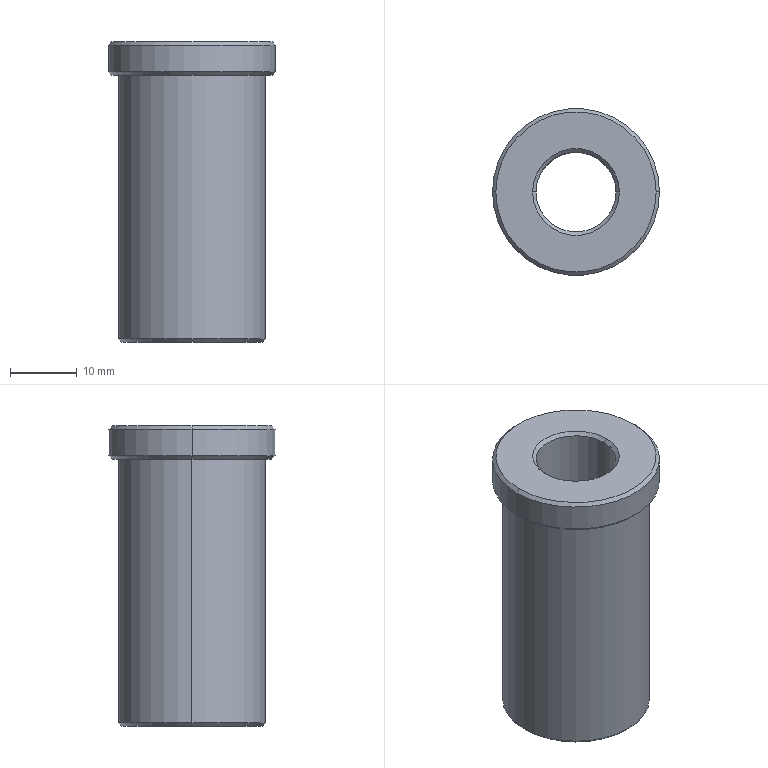Part | STEP file | 1 solid | 19 faces | box 25 x 25 x 45 mm | volume 12533 mm3 | cone 10 | cylinder 6 | plane 3 | commonest cylinder face diameters 12 x2 22 x2 25 x2
STEP:
#1=CARTESIAN_POINT('',(0.,0.,0.));
#2=DIRECTION('',(0.,0.,1.));
#3=DIRECTION('',(1.,0.,0.));
#4=AXIS2_PLACEMENT_3D('',#1,#2,#3);
#5=CARTESIAN_POINT('',(-10.5,0.,-40.));
#6=VERTEX_POINT('',#5);
#7=CARTESIAN_POINT('',(-11.,0.,-39.5));
#8=VERTEX_POINT('',#7);
#9=CARTESIAN_POINT('',(-10.5,0.,-40.));
#10=DIRECTION('',(-0.7071,0.,0.7071));
#11=VECTOR('',#10,1.);
#12=LINE('',#9,#11);
#13=CARTESIAN_POINT('',(0.,0.,-40.));
#14=DIRECTION('',(0.,0.,1.));
#15=DIRECTION('',(1.,0.,0.));
#16=AXIS2_PLACEMENT_3D('',#13,#14,#15);
#17=CONICAL_SURFACE('',#16,10.5,0.7854);
#18=CARTESIAN_POINT('',(3.142,0.));
#19=DIRECTION('',(0.,1.));
#20=VECTOR('',#19,1.);
#21=LINE('',#18,#20);
#22=(GEOMETRIC_REPRESENTATION_CONTEXT(2)PARAMETRIC_REPRESENTATION_CONTEXT()REPRESENTATION_CONTEXT('',''));
#23=DEFINITIONAL_REPRESENTATION('',(#21),#22);
#24=PCURVE('',#17,#23);
#25=CARTESIAN_POINT('',(0.,0.,-40.));
#26=DIRECTION('',(0.,0.,1.));
#27=DIRECTION('',(1.,0.,0.));
#28=AXIS2_PLACEMENT_3D('',#25,#26,#27);
#29=CONICAL_SURFACE('',#28,10.5,0.7854);
#30=CARTESIAN_POINT('',(3.142,0.));
#31=DIRECTION('',(0.,1.));
#32=VECTOR('',#31,1.);
#33=LINE('',#30,#32);
#34=(GEOMETRIC_REPRESENTATION_CONTEXT(2)PARAMETRIC_REPRESENTATION_CONTEXT()REPRESENTATION_CONTEXT('',''));
#35=DEFINITIONAL_REPRESENTATION('',(#33),#34);
#36=PCURVE('',#29,#35);
#37=SURFACE_CURVE('',#12,(#24,#36),.PCURVE_S1.);
#38=EDGE_CURVE('',#6,#8,#37,.T.);
#39=ORIENTED_EDGE('',*,*,#38,.F.);
#40=CARTESIAN_POINT('',(10.5,0.,-40.));
#41=VERTEX_POINT('',#40);
#42=CARTESIAN_POINT('',(0.,0.,-40.));
#43=DIRECTION('',(0.,0.,-1.));
#44=DIRECTION('',(-1.,0.,0.));
#45=AXIS2_PLACEMENT_3D('',#42,#43,#44);
#46=CIRCLE('',#45,10.5);
#47=CARTESIAN_POINT('',(9.425,0.));
#48=DIRECTION('',(-1.,0.));
#49=VECTOR('',#48,1.);
#50=LINE('',#47,#49);
#51=(GEOMETRIC_REPRESENTATION_CONTEXT(2)PARAMETRIC_REPRESENTATION_CONTEXT()REPRESENTATION_CONTEXT('',''));
#52=DEFINITIONAL_REPRESENTATION('',(#50),#51);
#53=PCURVE('',#17,#52);
#54=CARTESIAN_POINT('',(0.,0.,-40.));
#55=DIRECTION('',(0.,0.,-1.));
#56=DIRECTION('',(0.,-1.,0.));
#57=AXIS2_PLACEMENT_3D('',#54,#55,#56);
#58=PLANE('',#57);
#59=CARTESIAN_POINT('',(0.,0.));
#60=DIRECTION('',(0.,1.));
#61=AXIS2_PLACEMENT_2D('',#59,#60);
#62=CIRCLE('',#61,10.5);
#63=(GEOMETRIC_REPRESENTATION_CONTEXT(2)PARAMETRIC_REPRESENTATION_CONTEXT()REPRESENTATION_CONTEXT('',''));
#64=DEFINITIONAL_REPRESENTATION('',(#62),#63);
#65=PCURVE('',#58,#64);
#66=SURFACE_CURVE('',#46,(#53,#65),.PCURVE_S1.);
#67=EDGE_CURVE('',#41,#6,#66,.T.);
#68=ORIENTED_EDGE('',*,*,#67,.F.);
#69=CARTESIAN_POINT('',(11.,0.,-39.5));
#70=VERTEX_POINT('',#69);
#71=CARTESIAN_POINT('',(10.5,0.,-40.));
#72=DIRECTION('',(0.7071,0.,0.7071));
#73=VECTOR('',#72,1.);
#74=LINE('',#71,#73);
#75=CARTESIAN_POINT('',(6.283,0.));
#76=DIRECTION('',(0.,1.));
#77=VECTOR('',#76,1.);
#78=LINE('',#75,#77);
#79=(GEOMETRIC_REPRESENTATION_CONTEXT(2)PARAMETRIC_REPRESENTATION_CONTEXT()REPRESENTATION_CONTEXT('',''));
#80=DEFINITIONAL_REPRESENTATION('',(#78),#79);
#81=PCURVE('',#17,#80);
#82=CARTESIAN_POINT('',(0.,0.));
#83=DIRECTION('',(0.,1.));
#84=VECTOR('',#83,1.);
#85=LINE('',#82,#84);
#86=(GEOMETRIC_REPRESENTATION_CONTEXT(2)PARAMETRIC_REPRESENTATION_CONTEXT()REPRESENTATION_CONTEXT('',''));
#87=DEFINITIONAL_REPRESENTATION('',(#85),#86);
#88=PCURVE('',#29,#87);
#89=SURFACE_CURVE('',#74,(#81,#88),.PCURVE_S1.);
#90=EDGE_CURVE('',#41,#70,#89,.T.);
#91=ORIENTED_EDGE('',*,*,#90,.T.);
#92=CARTESIAN_POINT('',(0.,0.,-39.5));
#93=DIRECTION('',(0.,0.,1.));
#94=DIRECTION('',(-1.,0.,0.));
#95=AXIS2_PLACEMENT_3D('',#92,#93,#94);
#96=CIRCLE('',#95,11.);
#97=CARTESIAN_POINT('',(3.142,0.5));
#98=DIRECTION('',(1.,0.));
#99=VECTOR('',#98,1.);
#100=LINE('',#97,#99);
#101=(GEOMETRIC_REPRESENTATION_CONTEXT(2)PARAMETRIC_REPRESENTATION_CONTEXT()REPRESENTATION_CONTEXT('',''));
#102=DEFINITIONAL_REPRESENTATION('',(#100),#101);
#103=PCURVE('',#17,#102);
#104=CARTESIAN_POINT('',(0.,0.,-40.));
#105=DIRECTION('',(0.,0.,1.));
#106=DIRECTION('',(1.,0.,0.));
#107=AXIS2_PLACEMENT_3D('',#104,#105,#106);
#108=CYLINDRICAL_SURFACE('',#107,11.);
#109=CARTESIAN_POINT('',(3.142,0.5));
#110=DIRECTION('',(1.,0.));
#111=VECTOR('',#110,1.);
#112=LINE('',#109,#111);
#113=(GEOMETRIC_REPRESENTATION_CONTEXT(2)PARAMETRIC_REPRESENTATION_CONTEXT()REPRESENTATION_CONTEXT('',''));
#114=DEFINITIONAL_REPRESENTATION('',(#112),#113);
#115=PCURVE('',#108,#114);
#116=SURFACE_CURVE('',#96,(#103,#115),.PCURVE_S1.);
#117=EDGE_CURVE('',#8,#70,#116,.T.);
#118=ORIENTED_EDGE('',*,*,#117,.F.);
#119=EDGE_LOOP('',(#39,#68,#91,#118));
#120=FACE_BOUND('',#119,.T.);
#121=ADVANCED_FACE('',(#120),#17,.T.);
#122=CARTESIAN_POINT('',(-12.,0.,0.));
#123=VERTEX_POINT('',#122);
#124=CARTESIAN_POINT('',(-12.5,0.,0.5));
#125=VERTEX_POINT('',#124);
#126=CARTESIAN_POINT('',(-12.5,0.,0.5));
#127=DIRECTION('',(-0.7071,0.,0.7071));
#128=VECTOR('',#127,1.);
#129=LINE('',#126,#128);
#130=CARTESIAN_POINT('',(0.,0.,0.5));
#131=DIRECTION('',(0.,0.,1.));
#132=DIRECTION('',(1.,0.,0.));
#133=AXIS2_PLACEMENT_3D('',#130,#131,#132);
#134=CONICAL_SURFACE('',#133,12.5,0.7854);
#135=CARTESIAN_POINT('',(3.142,0.));
#136=DIRECTION('',(0.,1.));
#137=VECTOR('',#136,1.);
#138=LINE('',#135,#137);
#139=(GEOMETRIC_REPRESENTATION_CONTEXT(2)PARAMETRIC_REPRESENTATION_CONTEXT()REPRESENTATION_CONTEXT('',''));
#140=DEFINITIONAL_REPRESENTATION('',(#138),#139);
#141=PCURVE('',#134,#140);
#142=CARTESIAN_POINT('',(0.,0.,0.5));
#143=DIRECTION('',(0.,0.,1.));
#144=DIRECTION('',(1.,0.,0.));
#145=AXIS2_PLACEMENT_3D('',#142,#143,#144);
#146=CONICAL_SURFACE('',#145,12.5,0.7854);
#147=CARTESIAN_POINT('',(3.142,0.));
#148=DIRECTION('',(0.,1.));
#149=VECTOR('',#148,1.);
#150=LINE('',#147,#149);
#151=(GEOMETRIC_REPRESENTATION_CONTEXT(2)PARAMETRIC_REPRESENTATION_CONTEXT()REPRESENTATION_CONTEXT('',''));
#152=DEFINITIONAL_REPRESENTATION('',(#150),#151);
#153=PCURVE('',#146,#152);
#154=SURFACE_CURVE('',#129,(#141,#153),.PCURVE_S1.);
#155=EDGE_CURVE('',#123,#125,#154,.T.);
#156=ORIENTED_EDGE('',*,*,#155,.F.);
#157=CARTESIAN_POINT('',(12.,0.,0.));
#158=VERTEX_POINT('',#157);
#159=CARTESIAN_POINT('',(0.,0.,0.));
#160=DIRECTION('',(0.,0.,-1.));
#161=DIRECTION('',(1.,0.,0.));
#162=AXIS2_PLACEMENT_3D('',#159,#160,#161);
#163=CIRCLE('',#162,12.);
#164=CARTESIAN_POINT('',(6.283,-0.5));
#165=DIRECTION('',(-1.,0.));
#166=VECTOR('',#165,1.);
#167=LINE('',#164,#166);
#168=(GEOMETRIC_REPRESENTATION_CONTEXT(2)PARAMETRIC_REPRESENTATION_CONTEXT()REPRESENTATION_CONTEXT('',''));
#169=DEFINITIONAL_REPRESENTATION('',(#167),#168);
#170=PCURVE('',#134,#169);
#171=CARTESIAN_POINT('',(0.,0.,0.));
#172=DIRECTION('',(0.,0.,1.));
#173=DIRECTION('',(1.,0.,0.));
#174=AXIS2_PLACEMENT_3D('',#171,#172,#173);
#175=PLANE('',#174);
#176=CARTESIAN_POINT('',(12.,0.));
#177=CARTESIAN_POINT('',(12.,-20.785));
#178=CARTESIAN_POINT('',(-6.,-10.392));
#179=CARTESIAN_POINT('',(-24.,0.));
#180=CARTESIAN_POINT('',(-6.,10.392));
#181=CARTESIAN_POINT('',(12.,20.785));
#182=CARTESIAN_POINT('',(12.,0.));
#183=(BOUNDED_CURVE()B_SPLINE_CURVE(2,(#176,#177,#178,#179,#180,#181,#182),.UNSPECIFIED.,.T.,.F.)B_SPLINE_CURVE_WITH_KNOTS((1,2,2,2,2,1),(-2.094,0.,2.094,4.189,6.283,8.378),.UNSPECIFIED.)CURVE()GEOMETRIC_REPRESENTATION_ITEM()RATIONAL_B_SPLINE_CURVE((1.,0.5,1.,0.5,1.,0.5,1.))REPRESENTATION_ITEM(''));
#184=(GEOMETRIC_REPRESENTATION_CONTEXT(2)PARAMETRIC_REPRESENTATION_CONTEXT()REPRESENTATION_CONTEXT('',''));
#185=DEFINITIONAL_REPRESENTATION('',(#183),#184);
#186=PCURVE('',#175,#185);
#187=SURFACE_CURVE('',#163,(#170,#186),.PCURVE_S1.);
#188=EDGE_CURVE('',#158,#123,#187,.T.);
#189=ORIENTED_EDGE('',*,*,#188,.F.);
#190=CARTESIAN_POINT('',(12.5,0.,0.5));
#191=VERTEX_POINT('',#190);
#192=CARTESIAN_POINT('',(12.5,0.,0.5));
#193=DIRECTION('',(0.7071,0.,0.7071));
#194=VECTOR('',#193,1.);
#195=LINE('',#192,#194);
#196=CARTESIAN_POINT('',(6.283,0.));
#197=DIRECTION('',(0.,1.));
#198=VECTOR('',#197,1.);
#199=LINE('',#196,#198);
#200=(GEOMETRIC_REPRESENTATION_CONTEXT(2)PARAMETRIC_REPRESENTATION_CONTEXT()REPRESENTATION_CONTEXT('',''));
#201=DEFINITIONAL_REPRESENTATION('',(#199),#200);
#202=PCURVE('',#134,#201);
#203=CARTESIAN_POINT('',(0.,0.));
#204=DIRECTION('',(0.,1.));
#205=VECTOR('',#204,1.);
#206=LINE('',#203,#205);
#207=(GEOMETRIC_REPRESENTATION_CONTEXT(2)PARAMETRIC_REPRESENTATION_CONTEXT()REPRESENTATION_CONTEXT('',''));
#208=DEFINITIONAL_REPRESENTATION('',(#206),#207);
#209=PCURVE('',#146,#208);
#210=SURFACE_CURVE('',#195,(#202,#209),.PCURVE_S1.);
#211=EDGE_CURVE('',#158,#191,#210,.T.);
#212=ORIENTED_EDGE('',*,*,#211,.T.);
#213=CARTESIAN_POINT('',(0.,0.,0.5));
#214=DIRECTION('',(0.,0.,1.));
#215=DIRECTION('',(1.,0.,0.));
#216=AXIS2_PLACEMENT_3D('',#213,#214,#215);
#217=CIRCLE('',#216,12.5);
#218=CARTESIAN_POINT('',(0.,0.));
#219=DIRECTION('',(1.,0.));
#220=VECTOR('',#219,1.);
#221=LINE('',#218,#220);
#222=(GEOMETRIC_REPRESENTATION_CONTEXT(2)PARAMETRIC_REPRESENTATION_CONTEXT()REPRESENTATION_CONTEXT('',''));
#223=DEFINITIONAL_REPRESENTATION('',(#221),#222);
#224=PCURVE('',#134,#223);
#225=CARTESIAN_POINT('',(0.,0.,5.));
#226=DIRECTION('',(0.,0.,-1.));
#227=DIRECTION('',(-1.,0.,0.));
#228=AXIS2_PLACEMENT_3D('',#225,#226,#227);
#229=CYLINDRICAL_SURFACE('',#228,12.5);
#230=CARTESIAN_POINT('',(9.425,4.5));
#231=DIRECTION('',(-1.,0.));
#232=VECTOR('',#231,1.);
#233=LINE('',#230,#232);
#234=(GEOMETRIC_REPRESENTATION_CONTEXT(2)PARAMETRIC_REPRESENTATION_CONTEXT()REPRESENTATION_CONTEXT('',''));
#235=DEFINITIONAL_REPRESENTATION('',(#233),#234);
#236=PCURVE('',#229,#235);
#237=SURFACE_CURVE('',#217,(#224,#236),.PCURVE_S1.);
#238=EDGE_CURVE('',#125,#191,#237,.T.);
#239=ORIENTED_EDGE('',*,*,#238,.F.);
#240=EDGE_LOOP('',(#156,#189,#212,#239));
#241=FACE_BOUND('',#240,.T.);
#242=ADVANCED_FACE('',(#241),#134,.T.);
#243=CARTESIAN_POINT('',(-6.5,0.,5.));
#244=VERTEX_POINT('',#243);
#245=CARTESIAN_POINT('',(6.5,0.,5.));
#246=VERTEX_POINT('',#245);
#247=CARTESIAN_POINT('',(0.,0.,5.));
#248=DIRECTION('',(0.,0.,-1.));
#249=DIRECTION('',(1.,0.,0.));
#250=AXIS2_PLACEMENT_3D('',#247,#248,#249);
#251=CIRCLE('',#250,6.5);
#252=CARTESIAN_POINT('',(0.,0.,4.5));
#253=DIRECTION('',(0.,0.,1.));
#254=DIRECTION('',(1.,0.,0.));
#255=AXIS2_PLACEMENT_3D('',#252,#253,#254);
#256=CONICAL_SURFACE('',#255,6.,0.7854);
#257=CARTESIAN_POINT('',(6.283,0.5));
#258=DIRECTION('',(-1.,0.));
#259=VECTOR('',#258,1.);
#260=LINE('',#257,#259);
#261=(GEOMETRIC_REPRESENTATION_CONTEXT(2)PARAMETRIC_REPRESENTATION_CONTEXT()REPRESENTATION_CONTEXT('',''));
#262=DEFINITIONAL_REPRESENTATION('',(#260),#261);
#263=PCURVE('',#256,#262);
#264=CARTESIAN_POINT('',(0.,0.,5.));
#265=DIRECTION('',(0.,0.,1.));
#266=DIRECTION('',(1.,0.,0.));
#267=AXIS2_PLACEMENT_3D('',#264,#265,#266);
#268=PLANE('',#267);
#269=CARTESIAN_POINT('',(6.5,0.));
#270=CARTESIAN_POINT('',(6.5,-11.258));
#271=CARTESIAN_POINT('',(-3.25,-5.629));
#272=CARTESIAN_POINT('',(-13.,0.));
#273=CARTESIAN_POINT('',(-3.25,5.629));
#274=CARTESIAN_POINT('',(6.5,11.258));
#275=CARTESIAN_POINT('',(6.5,0.));
#276=(BOUNDED_CURVE()B_SPLINE_CURVE(2,(#269,#270,#271,#272,#273,#274,#275),.UNSPECIFIED.,.T.,.F.)B_SPLINE_CURVE_WITH_KNOTS((1,2,2,2,2,1),(-2.094,0.,2.094,4.189,6.283,8.378),.UNSPECIFIED.)CURVE()GEOMETRIC_REPRESENTATION_ITEM()RATIONAL_B_SPLINE_CURVE((1.,0.5,1.,0.5,1.,0.5,1.))REPRESENTATION_ITEM(''));
#277=(GEOMETRIC_REPRESENTATION_CONTEXT(2)PARAMETRIC_REPRESENTATION_CONTEXT()REPRESENTATION_CONTEXT('',''));
#278=DEFINITIONAL_REPRESENTATION('',(#276),#277);
#279=PCURVE('',#268,#278);
#280=SURFACE_CURVE('',#251,(#263,#279),.PCURVE_S1.);
#281=EDGE_CURVE('',#244,#246,#280,.T.);
#282=ORIENTED_EDGE('',*,*,#281,.T.);
#283=CARTESIAN_POINT('',(6.,0.,4.5));
#284=VERTEX_POINT('',#283);
#285=CARTESIAN_POINT('',(6.,0.,4.5));
#286=DIRECTION('',(0.7071,0.,0.7071));
#287=VECTOR('',#286,1.);
#288=LINE('',#285,#287);
#289=CARTESIAN_POINT('',(0.,0.));
#290=DIRECTION('',(0.,1.));
#291=VECTOR('',#290,1.);
#292=LINE('',#289,#291);
#293=(GEOMETRIC_REPRESENTATION_CONTEXT(2)PARAMETRIC_REPRESENTATION_CONTEXT()REPRESENTATION_CONTEXT('',''));
#294=DEFINITIONAL_REPRESENTATION('',(#292),#293);
#295=PCURVE('',#256,#294);
#296=CARTESIAN_POINT('',(0.,0.,4.5));
#297=DIRECTION('',(0.,0.,1.));
#298=DIRECTION('',(1.,0.,0.));
#299=AXIS2_PLACEMENT_3D('',#296,#297,#298);
#300=CONICAL_SURFACE('',#299,6.,0.7854);
#301=CARTESIAN_POINT('',(6.283,0.));
#302=DIRECTION('',(0.,1.));
#303=VECTOR('',#302,1.);
#304=LINE('',#301,#303);
#305=(GEOMETRIC_REPRESENTATION_CONTEXT(2)PARAMETRIC_REPRESENTATION_CONTEXT()REPRESENTATION_CONTEXT('',''));
#306=DEFINITIONAL_REPRESENTATION('',(#304),#305);
#307=PCURVE('',#300,#306);
#308=SURFACE_CURVE('',#288,(#295,#307),.PCURVE_S1.);
#309=EDGE_CURVE('',#284,#246,#308,.T.);
#310=ORIENTED_EDGE('',*,*,#309,.F.);
#311=CARTESIAN_POINT('',(-6.,0.,4.5));
#312=VERTEX_POINT('',#311);
#313=CARTESIAN_POINT('',(0.,0.,4.5));
#314=DIRECTION('',(0.,0.,1.));
#315=DIRECTION('',(1.,0.,0.));
#316=AXIS2_PLACEMENT_3D('',#313,#314,#315);
#317=CIRCLE('',#316,6.);
#318=CARTESIAN_POINT('',(0.,0.));
#319=DIRECTION('',(1.,0.));
#320=VECTOR('',#319,1.);
#321=LINE('',#318,#320);
#322=(GEOMETRIC_REPRESENTATION_CONTEXT(2)PARAMETRIC_REPRESENTATION_CONTEXT()REPRESENTATION_CONTEXT('',''));
#323=DEFINITIONAL_REPRESENTATION('',(#321),#322);
#324=PCURVE('',#256,#323);
#325=CARTESIAN_POINT('',(0.,0.,5.));
#326=DIRECTION('',(0.,0.,-1.));
#327=DIRECTION('',(-1.,0.,0.));
#328=AXIS2_PLACEMENT_3D('',#325,#326,#327);
#329=CYLINDRICAL_SURFACE('',#328,6.);
#330=CARTESIAN_POINT('',(3.142,0.5));
#331=DIRECTION('',(-1.,0.));
#332=VECTOR('',#331,1.);
#333=LINE('',#330,#332);
#334=(GEOMETRIC_REPRESENTATION_CONTEXT(2)PARAMETRIC_REPRESENTATION_CONTEXT()REPRESENTATION_CONTEXT('',''));
#335=DEFINITIONAL_REPRESENTATION('',(#333),#334);
#336=PCURVE('',#329,#335);
#337=SURFACE_CURVE('',#317,(#324,#336),.PCURVE_S1.);
#338=EDGE_CURVE('',#284,#312,#337,.T.);
#339=ORIENTED_EDGE('',*,*,#338,.T.);
#340=CARTESIAN_POINT('',(-6.,0.,4.5));
#341=DIRECTION('',(-0.7071,0.,0.7071));
#342=VECTOR('',#341,1.);
#343=LINE('',#340,#342);
#344=CARTESIAN_POINT('',(3.142,0.));
#345=DIRECTION('',(0.,1.));
#346=VECTOR('',#345,1.);
#347=LINE('',#344,#346);
#348=(GEOMETRIC_REPRESENTATION_CONTEXT(2)PARAMETRIC_REPRESENTATION_CONTEXT()REPRESENTATION_CONTEXT('',''));
#349=DEFINITIONAL_REPRESENTATION('',(#347),#348);
#350=PCURVE('',#256,#349);
#351=CARTESIAN_POINT('',(3.142,0.));
#352=DIRECTION('',(0.,1.));
#353=VECTOR('',#352,1.);
#354=LINE('',#351,#353);
#355=(GEOMETRIC_REPRESENTATION_CONTEXT(2)PARAMETRIC_REPRESENTATION_CONTEXT()REPRESENTATION_CONTEXT('',''));
#356=DEFINITIONAL_REPRESENTATION('',(#354),#355);
#357=PCURVE('',#300,#356);
#358=SURFACE_CURVE('',#343,(#350,#357),.PCURVE_S1.);
#359=EDGE_CURVE('',#312,#244,#358,.T.);
#360=ORIENTED_EDGE('',*,*,#359,.T.);
#361=EDGE_LOOP('',(#282,#310,#339,#360));
#362=FACE_BOUND('',#361,.F.);
#363=ADVANCED_FACE('',(#362),#256,.F.);
#364=CARTESIAN_POINT('',(6.5,0.,-40.));
#365=VERTEX_POINT('',#364);
#366=CARTESIAN_POINT('',(-6.5,0.,-40.));
#367=VERTEX_POINT('',#366);
#368=CARTESIAN_POINT('',(0.,0.,-40.));
#369=DIRECTION('',(0.,0.,1.));
#370=DIRECTION('',(-1.,0.,0.));
#371=AXIS2_PLACEMENT_3D('',#368,#369,#370);
#372=CIRCLE('',#371,6.5);
#373=CARTESIAN_POINT('',(0.,0.,-39.5));
#374=DIRECTION('',(0.,0.,-1.));
#375=DIRECTION('',(-1.,0.,0.));
#376=AXIS2_PLACEMENT_3D('',#373,#374,#375);
#377=CONICAL_SURFACE('',#376,6.,0.7854);
#378=CARTESIAN_POINT('',(6.283,0.5));
#379=DIRECTION('',(-1.,0.));
#380=VECTOR('',#379,1.);
#381=LINE('',#378,#380);
#382=(GEOMETRIC_REPRESENTATION_CONTEXT(2)PARAMETRIC_REPRESENTATION_CONTEXT()REPRESENTATION_CONTEXT('',''));
#383=DEFINITIONAL_REPRESENTATION('',(#381),#382);
#384=PCURVE('',#377,#383);
#385=CARTESIAN_POINT('',(0.,6.5));
#386=CARTESIAN_POINT('',(11.258,6.5));
#387=CARTESIAN_POINT('',(5.629,-3.25));
#388=CARTESIAN_POINT('',(0.,-13.));
#389=CARTESIAN_POINT('',(-5.629,-3.25));
#390=CARTESIAN_POINT('',(-11.258,6.5));
#391=CARTESIAN_POINT('',(0.,6.5));
#392=(BOUNDED_CURVE()B_SPLINE_CURVE(2,(#385,#386,#387,#388,#389,#390,#391),.UNSPECIFIED.,.T.,.F.)B_SPLINE_CURVE_WITH_KNOTS((1,2,2,2,2,1),(-2.094,0.,2.094,4.189,6.283,8.378),.UNSPECIFIED.)CURVE()GEOMETRIC_REPRESENTATION_ITEM()RATIONAL_B_SPLINE_CURVE((1.,0.5,1.,0.5,1.,0.5,1.))REPRESENTATION_ITEM(''));
#393=(GEOMETRIC_REPRESENTATION_CONTEXT(2)PARAMETRIC_REPRESENTATION_CONTEXT()REPRESENTATION_CONTEXT('',''));
#394=DEFINITIONAL_REPRESENTATION('',(#392),#393);
#395=PCURVE('',#58,#394);
#396=SURFACE_CURVE('',#372,(#384,#395),.PCURVE_S1.);
#397=EDGE_CURVE('',#365,#367,#396,.T.);
#398=ORIENTED_EDGE('',*,*,#397,.T.);
#399=CARTESIAN_POINT('',(-6.,0.,-39.5));
#400=VERTEX_POINT('',#399);
#401=CARTESIAN_POINT('',(-6.,0.,-39.5));
#402=DIRECTION('',(-0.7071,0.,-0.7071));
#403=VECTOR('',#402,1.);
#404=LINE('',#401,#403);
#405=CARTESIAN_POINT('',(0.,0.));
#406=DIRECTION('',(0.,1.));
#407=VECTOR('',#406,1.);
#408=LINE('',#405,#407);
#409=(GEOMETRIC_REPRESENTATION_CONTEXT(2)PARAMETRIC_REPRESENTATION_CONTEXT()REPRESENTATION_CONTEXT('',''));
#410=DEFINITIONAL_REPRESENTATION('',(#408),#409);
#411=PCURVE('',#377,#410);
#412=CARTESIAN_POINT('',(0.,0.,-39.5));
#413=DIRECTION('',(0.,0.,-1.));
#414=DIRECTION('',(-1.,0.,0.));
#415=AXIS2_PLACEMENT_3D('',#412,#413,#414);
#416=CONICAL_SURFACE('',#415,6.,0.7854);
#417=CARTESIAN_POINT('',(6.283,0.));
#418=DIRECTION('',(0.,1.));
#419=VECTOR('',#418,1.);
#420=LINE('',#417,#419);
#421=(GEOMETRIC_REPRESENTATION_CONTEXT(2)PARAMETRIC_REPRESENTATION_CONTEXT()REPRESENTATION_CONTEXT('',''));
#422=DEFINITIONAL_REPRESENTATION('',(#420),#421);
#423=PCURVE('',#416,#422);
#424=SURFACE_CURVE('',#404,(#411,#423),.PCURVE_S1.);
#425=EDGE_CURVE('',#400,#367,#424,.T.);
#426=ORIENTED_EDGE('',*,*,#425,.F.);
#427=CARTESIAN_POINT('',(6.,0.,-39.5));
#428=VERTEX_POINT('',#427);
#429=CARTESIAN_POINT('',(0.,0.,-39.5));
#430=DIRECTION('',(0.,0.,-1.));
#431=DIRECTION('',(-1.,0.,0.));
#432=AXIS2_PLACEMENT_3D('',#429,#430,#431);
#433=CIRCLE('',#432,6.);
#434=CARTESIAN_POINT('',(0.,0.));
#435=DIRECTION('',(1.,0.));
#436=VECTOR('',#435,1.);
#437=LINE('',#434,#436);
#438=(GEOMETRIC_REPRESENTATION_CONTEXT(2)PARAMETRIC_REPRESENTATION_CONTEXT()REPRESENTATION_CONTEXT('',''));
#439=DEFINITIONAL_REPRESENTATION('',(#437),#438);
#440=PCURVE('',#377,#439);
#441=CARTESIAN_POINT('',(0.,44.5));
#442=DIRECTION('',(1.,0.));
#443=VECTOR('',#442,1.);
#444=LINE('',#441,#443);
#445=(GEOMETRIC_REPRESENTATION_CONTEXT(2)PARAMETRIC_REPRESENTATION_CONTEXT()REPRESENTATION_CONTEXT('',''));
#446=DEFINITIONAL_REPRESENTATION('',(#444),#445);
#447=PCURVE('',#329,#446);
#448=SURFACE_CURVE('',#433,(#440,#447),.PCURVE_S1.);
#449=EDGE_CURVE('',#400,#428,#448,.T.);
#450=ORIENTED_EDGE('',*,*,#449,.T.);
#451=CARTESIAN_POINT('',(6.,0.,-39.5));
#452=DIRECTION('',(0.7071,0.,-0.7071));
#453=VECTOR('',#452,1.);
#454=LINE('',#451,#453);
#455=CARTESIAN_POINT('',(3.142,0.));
#456=DIRECTION('',(0.,1.));
#457=VECTOR('',#456,1.);
#458=LINE('',#455,#457);
#459=(GEOMETRIC_REPRESENTATION_CONTEXT(2)PARAMETRIC_REPRESENTATION_CONTEXT()REPRESENTATION_CONTEXT('',''));
#460=DEFINITIONAL_REPRESENTATION('',(#458),#459);
#461=PCURVE('',#377,#460);
#462=CARTESIAN_POINT('',(3.142,0.));
#463=DIRECTION('',(0.,1.));
#464=VECTOR('',#463,1.);
#465=LINE('',#462,#464);
#466=(GEOMETRIC_REPRESENTATION_CONTEXT(2)PARAMETRIC_REPRESENTATION_CONTEXT()REPRESENTATION_CONTEXT('',''));
#467=DEFINITIONAL_REPRESENTATION('',(#465),#466);
#468=PCURVE('',#416,#467);
#469=SURFACE_CURVE('',#454,(#461,#468),.PCURVE_S1.);
#470=EDGE_CURVE('',#428,#365,#469,.T.);
#471=ORIENTED_EDGE('',*,*,#470,.T.);
#472=EDGE_LOOP('',(#398,#426,#450,#471));
#473=FACE_BOUND('',#472,.F.);
#474=ADVANCED_FACE('',(#473),#377,.F.);
#475=CARTESIAN_POINT('',(12.,0.,5.));
#476=VERTEX_POINT('',#475);
#477=CARTESIAN_POINT('',(12.5,0.,4.5));
#478=VERTEX_POINT('',#477);
#479=CARTESIAN_POINT('',(12.,0.,5.));
#480=DIRECTION('',(0.7071,0.,-0.7071));
#481=VECTOR('',#480,1.);
#482=LINE('',#479,#481);
#483=CARTESIAN_POINT('',(0.,0.,5.));
#484=DIRECTION('',(0.,0.,-1.));
#485=DIRECTION('',(-1.,0.,0.));
#486=AXIS2_PLACEMENT_3D('',#483,#484,#485);
#487=CONICAL_SURFACE('',#486,12.,0.7854);
#488=CARTESIAN_POINT('',(3.142,0.));
#489=DIRECTION('',(0.,1.));
#490=VECTOR('',#489,1.);
#491=LINE('',#488,#490);
#492=(GEOMETRIC_REPRESENTATION_CONTEXT(2)PARAMETRIC_REPRESENTATION_CONTEXT()REPRESENTATION_CONTEXT('',''));
#493=DEFINITIONAL_REPRESENTATION('',(#491),#492);
#494=PCURVE('',#487,#493);
#495=CARTESIAN_POINT('',(0.,0.,5.));
#496=DIRECTION('',(0.,0.,-1.));
#497=DIRECTION('',(-1.,0.,0.));
#498=AXIS2_PLACEMENT_3D('',#495,#496,#497);
#499=CONICAL_SURFACE('',#498,12.,0.7854);
#500=CARTESIAN_POINT('',(3.142,0.));
#501=DIRECTION('',(0.,1.));
#502=VECTOR('',#501,1.);
#503=LINE('',#500,#502);
#504=(GEOMETRIC_REPRESENTATION_CONTEXT(2)PARAMETRIC_REPRESENTATION_CONTEXT()REPRESENTATION_CONTEXT('',''));
#505=DEFINITIONAL_REPRESENTATION('',(#503),#504);
#506=PCURVE('',#499,#505);
#507=SURFACE_CURVE('',#482,(#494,#506),.PCURVE_S1.);
#508=EDGE_CURVE('',#476,#478,#507,.T.);
#509=ORIENTED_EDGE('',*,*,#508,.F.);
#510=CARTESIAN_POINT('',(-12.,0.,5.));
#511=VERTEX_POINT('',#510);
#512=CARTESIAN_POINT('',(0.,0.,5.));
#513=DIRECTION('',(0.,0.,1.));
#514=DIRECTION('',(1.,0.,0.));
#515=AXIS2_PLACEMENT_3D('',#512,#513,#514);
#516=CIRCLE('',#515,12.);
#517=CARTESIAN_POINT('',(9.425,0.));
#518=DIRECTION('',(-1.,0.));
#519=VECTOR('',#518,1.);
#520=LINE('',#517,#519);
#521=(GEOMETRIC_REPRESENTATION_CONTEXT(2)PARAMETRIC_REPRESENTATION_CONTEXT()REPRESENTATION_CONTEXT('',''));
#522=DEFINITIONAL_REPRESENTATION('',(#520),#521);
#523=PCURVE('',#487,#522);
#524=CARTESIAN_POINT('',(0.,0.));
#525=DIRECTION('',(1.,0.));
#526=AXIS2_PLACEMENT_2D('',#524,#525);
#527=CIRCLE('',#526,12.);
#528=(GEOMETRIC_REPRESENTATION_CONTEXT(2)PARAMETRIC_REPRESENTATION_CONTEXT()REPRESENTATION_CONTEXT('',''));
#529=DEFINITIONAL_REPRESENTATION('',(#527),#528);
#530=PCURVE('',#268,#529);
#531=SURFACE_CURVE('',#516,(#523,#530),.PCURVE_S1.);
#532=EDGE_CURVE('',#511,#476,#531,.T.);
#533=ORIENTED_EDGE('',*,*,#532,.F.);
#534=CARTESIAN_POINT('',(-12.5,0.,4.5));
#535=VERTEX_POINT('',#534);
#536=CARTESIAN_POINT('',(-12.,0.,5.));
#537=DIRECTION('',(-0.7071,0.,-0.7071));
#538=VECTOR('',#537,1.);
#539=LINE('',#536,#538);
#540=CARTESIAN_POINT('',(6.283,0.));
#541=DIRECTION('',(0.,1.));
#542=VECTOR('',#541,1.);
#543=LINE('',#540,#542);
#544=(GEOMETRIC_REPRESENTATION_CONTEXT(2)PARAMETRIC_REPRESENTATION_CONTEXT()REPRESENTATION_CONTEXT('',''));
#545=DEFINITIONAL_REPRESENTATION('',(#543),#544);
#546=PCURVE('',#487,#545);
#547=CARTESIAN_POINT('',(0.,0.));
#548=DIRECTION('',(0.,1.));
#549=VECTOR('',#548,1.);
#550=LINE('',#547,#549);
#551=(GEOMETRIC_REPRESENTATION_CONTEXT(2)PARAMETRIC_REPRESENTATION_CONTEXT()REPRESENTATION_CONTEXT('',''));
#552=DEFINITIONAL_REPRESENTATION('',(#550),#551);
#553=PCURVE('',#499,#552);
#554=SURFACE_CURVE('',#539,(#546,#553),.PCURVE_S1.);
#555=EDGE_CURVE('',#511,#535,#554,.T.);
#556=ORIENTED_EDGE('',*,*,#555,.T.);
#557=CARTESIAN_POINT('',(0.,0.,4.5));
#558=DIRECTION('',(0.,0.,-1.));
#559=DIRECTION('',(1.,0.,0.));
#560=AXIS2_PLACEMENT_3D('',#557,#558,#559);
#561=CIRCLE('',#560,12.5);
#562=CARTESIAN_POINT('',(3.142,0.5));
#563=DIRECTION('',(1.,0.));
#564=VECTOR('',#563,1.);
#565=LINE('',#562,#564);
#566=(GEOMETRIC_REPRESENTATION_CONTEXT(2)PARAMETRIC_REPRESENTATION_CONTEXT()REPRESENTATION_CONTEXT('',''));
#567=DEFINITIONAL_REPRESENTATION('',(#565),#566);
#568=PCURVE('',#487,#567);
#569=CARTESIAN_POINT('',(3.142,0.5));
#570=DIRECTION('',(1.,0.));
#571=VECTOR('',#570,1.);
#572=LINE('',#569,#571);
#573=(GEOMETRIC_REPRESENTATION_CONTEXT(2)PARAMETRIC_REPRESENTATION_CONTEXT()REPRESENTATION_CONTEXT('',''));
#574=DEFINITIONAL_REPRESENTATION('',(#572),#573);
#575=PCURVE('',#229,#574);
#576=SURFACE_CURVE('',#561,(#568,#575),.PCURVE_S1.);
#577=EDGE_CURVE('',#478,#535,#576,.T.);
#578=ORIENTED_EDGE('',*,*,#577,.F.);
#579=EDGE_LOOP('',(#509,#533,#556,#578));
#580=FACE_BOUND('',#579,.T.);
#581=ADVANCED_FACE('',(#580),#487,.T.);
#582=CARTESIAN_POINT('',(-11.,0.,0.));
#583=VERTEX_POINT('',#582);
#584=CARTESIAN_POINT('',(-11.,0.,-40.));
#585=DIRECTION('',(0.,0.,1.));
#586=VECTOR('',#585,1.);
#587=LINE('',#584,#586);
#588=CARTESIAN_POINT('',(3.142,0.));
#589=DIRECTION('',(0.,1.));
#590=VECTOR('',#589,1.);
#591=LINE('',#588,#590);
#592=(GEOMETRIC_REPRESENTATION_CONTEXT(2)PARAMETRIC_REPRESENTATION_CONTEXT()REPRESENTATION_CONTEXT('',''));
#593=DEFINITIONAL_REPRESENTATION('',(#591),#592);
#594=PCURVE('',#108,#593);
#595=CARTESIAN_POINT('',(0.,0.,-40.));
#596=DIRECTION('',(0.,0.,1.));
#597=DIRECTION('',(1.,0.,0.));
#598=AXIS2_PLACEMENT_3D('',#595,#596,#597);
#599=CYLINDRICAL_SURFACE('',#598,11.);
#600=CARTESIAN_POINT('',(3.142,0.));
#601=DIRECTION('',(0.,1.));
#602=VECTOR('',#601,1.);
#603=LINE('',#600,#602);
#604=(GEOMETRIC_REPRESENTATION_CONTEXT(2)PARAMETRIC_REPRESENTATION_CONTEXT()REPRESENTATION_CONTEXT('',''));
#605=DEFINITIONAL_REPRESENTATION('',(#603),#604);
#606=PCURVE('',#599,#605);
#607=SURFACE_CURVE('',#587,(#594,#606),.PCURVE_S1.);
#608=EDGE_CURVE('',#8,#583,#607,.T.);
#609=ORIENTED_EDGE('',*,*,#608,.F.);
#610=ORIENTED_EDGE('',*,*,#117,.T.);
#611=CARTESIAN_POINT('',(11.,0.,0.));
#612=VERTEX_POINT('',#611);
#613=CARTESIAN_POINT('',(11.,0.,-40.));
#614=DIRECTION('',(0.,0.,1.));
#615=VECTOR('',#614,1.);
#616=LINE('',#613,#615);
#617=CARTESIAN_POINT('',(6.283,0.));
#618=DIRECTION('',(0.,1.));
#619=VECTOR('',#618,1.);
#620=LINE('',#617,#619);
#621=(GEOMETRIC_REPRESENTATION_CONTEXT(2)PARAMETRIC_REPRESENTATION_CONTEXT()REPRESENTATION_CONTEXT('',''));
#622=DEFINITIONAL_REPRESENTATION('',(#620),#621);
#623=PCURVE('',#108,#622);
#624=CARTESIAN_POINT('',(0.,0.));
#625=DIRECTION('',(0.,1.));
#626=VECTOR('',#625,1.);
#627=LINE('',#624,#626);
#628=(GEOMETRIC_REPRESENTATION_CONTEXT(2)PARAMETRIC_REPRESENTATION_CONTEXT()REPRESENTATION_CONTEXT('',''));
#629=DEFINITIONAL_REPRESENTATION('',(#627),#628);
#630=PCURVE('',#599,#629);
#631=SURFACE_CURVE('',#616,(#623,#630),.PCURVE_S1.);
#632=EDGE_CURVE('',#70,#612,#631,.T.);
#633=ORIENTED_EDGE('',*,*,#632,.T.);
#634=CARTESIAN_POINT('',(0.,0.,0.));
#635=DIRECTION('',(0.,0.,-1.));
#636=DIRECTION('',(-1.,0.,0.));
#637=AXIS2_PLACEMENT_3D('',#634,#635,#636);
#638=CIRCLE('',#637,11.);
#639=CARTESIAN_POINT('',(9.425,40.));
#640=DIRECTION('',(-1.,0.));
#641=VECTOR('',#640,1.);
#642=LINE('',#639,#641);
#643=(GEOMETRIC_REPRESENTATION_CONTEXT(2)PARAMETRIC_REPRESENTATION_CONTEXT()REPRESENTATION_CONTEXT('',''));
#644=DEFINITIONAL_REPRESENTATION('',(#642),#643);
#645=PCURVE('',#108,#644);
#646=CARTESIAN_POINT('',(-11.,0.));
#647=CARTESIAN_POINT('',(-11.,19.053));
#648=CARTESIAN_POINT('',(5.5,9.526));
#649=CARTESIAN_POINT('',(22.,0.));
#650=CARTESIAN_POINT('',(5.5,-9.526));
#651=CARTESIAN_POINT('',(-11.,-19.053));
#652=CARTESIAN_POINT('',(-11.,0.));
#653=(BOUNDED_CURVE()B_SPLINE_CURVE(2,(#646,#647,#648,#649,#650,#651,#652),.UNSPECIFIED.,.T.,.F.)B_SPLINE_CURVE_WITH_KNOTS((1,2,2,2,2,1),(-2.094,0.,2.094,4.189,6.283,8.378),.UNSPECIFIED.)CURVE()GEOMETRIC_REPRESENTATION_ITEM()RATIONAL_B_SPLINE_CURVE((1.,0.5,1.,0.5,1.,0.5,1.))REPRESENTATION_ITEM(''));
#654=(GEOMETRIC_REPRESENTATION_CONTEXT(2)PARAMETRIC_REPRESENTATION_CONTEXT()REPRESENTATION_CONTEXT('',''));
#655=DEFINITIONAL_REPRESENTATION('',(#653),#654);
#656=PCURVE('',#175,#655);
#657=SURFACE_CURVE('',#638,(#645,#656),.PCURVE_S1.);
#658=EDGE_CURVE('',#612,#583,#657,.T.);
#659=ORIENTED_EDGE('',*,*,#658,.T.);
#660=EDGE_LOOP('',(#609,#610,#633,#659));
#661=FACE_BOUND('',#660,.T.);
#662=ADVANCED_FACE('',(#661),#108,.T.);
#663=CARTESIAN_POINT('',(0.,0.,-40.));
#664=DIRECTION('',(0.,0.,1.));
#665=DIRECTION('',(-1.,0.,0.));
#666=AXIS2_PLACEMENT_3D('',#663,#664,#665);
#667=CIRCLE('',#666,6.5);
#668=CARTESIAN_POINT('',(0.,6.5));
#669=CARTESIAN_POINT('',(11.258,6.5));
#670=CARTESIAN_POINT('',(5.629,-3.25));
#671=CARTESIAN_POINT('',(0.,-13.));
#672=CARTESIAN_POINT('',(-5.629,-3.25));
#673=CARTESIAN_POINT('',(-11.258,6.5));
#674=CARTESIAN_POINT('',(0.,6.5));
#675=(BOUNDED_CURVE()B_SPLINE_CURVE(2,(#668,#669,#670,#671,#672,#673,#674),.UNSPECIFIED.,.T.,.F.)B_SPLINE_CURVE_WITH_KNOTS((1,2,2,2,2,1),(-2.094,0.,2.094,4.189,6.283,8.378),.UNSPECIFIED.)CURVE()GEOMETRIC_REPRESENTATION_ITEM()RATIONAL_B_SPLINE_CURVE((1.,0.5,1.,0.5,1.,0.5,1.))REPRESENTATION_ITEM(''));
#676=(GEOMETRIC_REPRESENTATION_CONTEXT(2)PARAMETRIC_REPRESENTATION_CONTEXT()REPRESENTATION_CONTEXT('',''));
#677=DEFINITIONAL_REPRESENTATION('',(#675),#676);
#678=PCURVE('',#58,#677);
#679=CARTESIAN_POINT('',(6.283,0.5));
#680=DIRECTION('',(-1.,0.));
#681=VECTOR('',#680,1.);
#682=LINE('',#679,#681);
#683=(GEOMETRIC_REPRESENTATION_CONTEXT(2)PARAMETRIC_REPRESENTATION_CONTEXT()REPRESENTATION_CONTEXT('',''));
#684=DEFINITIONAL_REPRESENTATION('',(#682),#683);
#685=PCURVE('',#416,#684);
#686=SURFACE_CURVE('',#667,(#678,#685),.PCURVE_S1.);
#687=EDGE_CURVE('',#367,#365,#686,.T.);
#688=ORIENTED_EDGE('',*,*,#687,.T.);
#689=ORIENTED_EDGE('',*,*,#397,.T.);
#690=EDGE_LOOP('',(#688,#689));
#691=FACE_BOUND('',#690,.T.);
#692=ORIENTED_EDGE('',*,*,#67,.T.);
#693=CARTESIAN_POINT('',(0.,0.,-40.));
#694=DIRECTION('',(0.,0.,-1.));
#695=DIRECTION('',(-1.,0.,0.));
#696=AXIS2_PLACEMENT_3D('',#693,#694,#695);
#697=CIRCLE('',#696,10.5);
#698=CARTESIAN_POINT('',(0.,0.));
#699=DIRECTION('',(0.,1.));
#700=AXIS2_PLACEMENT_2D('',#698,#699);
#701=CIRCLE('',#700,10.5);
#702=(GEOMETRIC_REPRESENTATION_CONTEXT(2)PARAMETRIC_REPRESENTATION_CONTEXT()REPRESENTATION_CONTEXT('',''));
#703=DEFINITIONAL_REPRESENTATION('',(#701),#702);
#704=PCURVE('',#58,#703);
#705=CARTESIAN_POINT('',(3.142,0.));
#706=DIRECTION('',(-1.,0.));
#707=VECTOR('',#706,1.);
#708=LINE('',#705,#707);
#709=(GEOMETRIC_REPRESENTATION_CONTEXT(2)PARAMETRIC_REPRESENTATION_CONTEXT()REPRESENTATION_CONTEXT('',''));
#710=DEFINITIONAL_REPRESENTATION('',(#708),#709);
#711=PCURVE('',#29,#710);
#712=SURFACE_CURVE('',#697,(#704,#711),.PCURVE_S1.);
#713=EDGE_CURVE('',#6,#41,#712,.T.);
#714=ORIENTED_EDGE('',*,*,#713,.T.);
#715=EDGE_LOOP('',(#692,#714));
#716=FACE_BOUND('',#715,.T.);
#717=ADVANCED_FACE('',(#691,#716),#58,.T.);
#718=ORIENTED_EDGE('',*,*,#449,.F.);
#719=CARTESIAN_POINT('',(-6.,0.,5.));
#720=DIRECTION('',(0.,0.,-1.));
#721=VECTOR('',#720,1.);
#722=LINE('',#719,#721);
#723=CARTESIAN_POINT('',(0.,0.));
#724=DIRECTION('',(0.,1.));
#725=VECTOR('',#724,1.);
#726=LINE('',#723,#725);
#727=(GEOMETRIC_REPRESENTATION_CONTEXT(2)PARAMETRIC_REPRESENTATION_CONTEXT()REPRESENTATION_CONTEXT('',''));
#728=DEFINITIONAL_REPRESENTATION('',(#726),#727);
#729=PCURVE('',#329,#728);
#730=CARTESIAN_POINT('',(0.,0.,5.));
#731=DIRECTION('',(0.,0.,-1.));
#732=DIRECTION('',(-1.,0.,0.));
#733=AXIS2_PLACEMENT_3D('',#730,#731,#732);
#734=CYLINDRICAL_SURFACE('',#733,6.);
#735=CARTESIAN_POINT('',(6.283,0.));
#736=DIRECTION('',(0.,1.));
#737=VECTOR('',#736,1.);
#738=LINE('',#735,#737);
#739=(GEOMETRIC_REPRESENTATION_CONTEXT(2)PARAMETRIC_REPRESENTATION_CONTEXT()REPRESENTATION_CONTEXT('',''));
#740=DEFINITIONAL_REPRESENTATION('',(#738),#739);
#741=PCURVE('',#734,#740);
#742=SURFACE_CURVE('',#722,(#729,#741),.PCURVE_S1.);
#743=EDGE_CURVE('',#312,#400,#742,.T.);
#744=ORIENTED_EDGE('',*,*,#743,.F.);
#745=ORIENTED_EDGE('',*,*,#338,.F.);
#746=CARTESIAN_POINT('',(6.,0.,5.));
#747=DIRECTION('',(0.,0.,-1.));
#748=VECTOR('',#747,1.);
#749=LINE('',#746,#748);
#750=CARTESIAN_POINT('',(3.142,0.));
#751=DIRECTION('',(0.,1.));
#752=VECTOR('',#751,1.);
#753=LINE('',#750,#752);
#754=(GEOMETRIC_REPRESENTATION_CONTEXT(2)PARAMETRIC_REPRESENTATION_CONTEXT()REPRESENTATION_CONTEXT('',''));
#755=DEFINITIONAL_REPRESENTATION('',(#753),#754);
#756=PCURVE('',#329,#755);
#757=CARTESIAN_POINT('',(3.142,0.));
#758=DIRECTION('',(0.,1.));
#759=VECTOR('',#758,1.);
#760=LINE('',#757,#759);
#761=(GEOMETRIC_REPRESENTATION_CONTEXT(2)PARAMETRIC_REPRESENTATION_CONTEXT()REPRESENTATION_CONTEXT('',''));
#762=DEFINITIONAL_REPRESENTATION('',(#760),#761);
#763=PCURVE('',#734,#762);
#764=SURFACE_CURVE('',#749,(#756,#763),.PCURVE_S1.);
#765=EDGE_CURVE('',#284,#428,#764,.T.);
#766=ORIENTED_EDGE('',*,*,#765,.T.);
#767=EDGE_LOOP('',(#718,#744,#745,#766));
#768=FACE_BOUND('',#767,.F.);
#769=ADVANCED_FACE('',(#768),#329,.F.);
#770=CARTESIAN_POINT('',(12.5,0.,5.));
#771=DIRECTION('',(0.,0.,-1.));
#772=VECTOR('',#771,1.);
#773=LINE('',#770,#772);
#774=CARTESIAN_POINT('',(3.142,0.));
#775=DIRECTION('',(0.,1.));
#776=VECTOR('',#775,1.);
#777=LINE('',#774,#776);
#778=(GEOMETRIC_REPRESENTATION_CONTEXT(2)PARAMETRIC_REPRESENTATION_CONTEXT()REPRESENTATION_CONTEXT('',''));
#779=DEFINITIONAL_REPRESENTATION('',(#777),#778);
#780=PCURVE('',#229,#779);
#781=CARTESIAN_POINT('',(0.,0.,5.));
#782=DIRECTION('',(0.,0.,-1.));
#783=DIRECTION('',(-1.,0.,0.));
#784=AXIS2_PLACEMENT_3D('',#781,#782,#783);
#785=CYLINDRICAL_SURFACE('',#784,12.5);
#786=CARTESIAN_POINT('',(3.142,0.));
#787=DIRECTION('',(0.,1.));
#788=VECTOR('',#787,1.);
#789=LINE('',#786,#788);
#790=(GEOMETRIC_REPRESENTATION_CONTEXT(2)PARAMETRIC_REPRESENTATION_CONTEXT()REPRESENTATION_CONTEXT('',''));
#791=DEFINITIONAL_REPRESENTATION('',(#789),#790);
#792=PCURVE('',#785,#791);
#793=SURFACE_CURVE('',#773,(#780,#792),.PCURVE_S1.);
#794=EDGE_CURVE('',#478,#191,#793,.T.);
#795=ORIENTED_EDGE('',*,*,#794,.F.);
#796=ORIENTED_EDGE('',*,*,#577,.T.);
#797=CARTESIAN_POINT('',(-12.5,0.,5.));
#798=DIRECTION('',(0.,0.,-1.));
#799=VECTOR('',#798,1.);
#800=LINE('',#797,#799);
#801=CARTESIAN_POINT('',(6.283,0.));
#802=DIRECTION('',(0.,1.));
#803=VECTOR('',#802,1.);
#804=LINE('',#801,#803);
#805=(GEOMETRIC_REPRESENTATION_CONTEXT(2)PARAMETRIC_REPRESENTATION_CONTEXT()REPRESENTATION_CONTEXT('',''));
#806=DEFINITIONAL_REPRESENTATION('',(#804),#805);
#807=PCURVE('',#229,#806);
#808=CARTESIAN_POINT('',(0.,0.));
#809=DIRECTION('',(0.,1.));
#810=VECTOR('',#809,1.);
#811=LINE('',#808,#810);
#812=(GEOMETRIC_REPRESENTATION_CONTEXT(2)PARAMETRIC_REPRESENTATION_CONTEXT()REPRESENTATION_CONTEXT('',''));
#813=DEFINITIONAL_REPRESENTATION('',(#811),#812);
#814=PCURVE('',#785,#813);
#815=SURFACE_CURVE('',#800,(#807,#814),.PCURVE_S1.);
#816=EDGE_CURVE('',#535,#125,#815,.T.);
#817=ORIENTED_EDGE('',*,*,#816,.T.);
#818=ORIENTED_EDGE('',*,*,#238,.T.);
#819=EDGE_LOOP('',(#795,#796,#817,#818));
#820=FACE_BOUND('',#819,.T.);
#821=ADVANCED_FACE('',(#820),#229,.T.);
#822=ORIENTED_EDGE('',*,*,#658,.F.);
#823=CARTESIAN_POINT('',(0.,0.,0.));
#824=DIRECTION('',(0.,0.,-1.));
#825=DIRECTION('',(-1.,0.,0.));
#826=AXIS2_PLACEMENT_3D('',#823,#824,#825);
#827=CIRCLE('',#826,11.);
#828=CARTESIAN_POINT('',(-11.,0.));
#829=CARTESIAN_POINT('',(-11.,19.053));
#830=CARTESIAN_POINT('',(5.5,9.526));
#831=CARTESIAN_POINT('',(22.,0.));
#832=CARTESIAN_POINT('',(5.5,-9.526));
#833=CARTESIAN_POINT('',(-11.,-19.053));
#834=CARTESIAN_POINT('',(-11.,0.));
#835=(BOUNDED_CURVE()B_SPLINE_CURVE(2,(#828,#829,#830,#831,#832,#833,#834),.UNSPECIFIED.,.T.,.F.)B_SPLINE_CURVE_WITH_KNOTS((1,2,2,2,2,1),(-2.094,0.,2.094,4.189,6.283,8.378),.UNSPECIFIED.)CURVE()GEOMETRIC_REPRESENTATION_ITEM()RATIONAL_B_SPLINE_CURVE((1.,0.5,1.,0.5,1.,0.5,1.))REPRESENTATION_ITEM(''));
#836=(GEOMETRIC_REPRESENTATION_CONTEXT(2)PARAMETRIC_REPRESENTATION_CONTEXT()REPRESENTATION_CONTEXT('',''));
#837=DEFINITIONAL_REPRESENTATION('',(#835),#836);
#838=PCURVE('',#175,#837);
#839=CARTESIAN_POINT('',(3.142,40.));
#840=DIRECTION('',(-1.,0.));
#841=VECTOR('',#840,1.);
#842=LINE('',#839,#841);
#843=(GEOMETRIC_REPRESENTATION_CONTEXT(2)PARAMETRIC_REPRESENTATION_CONTEXT()REPRESENTATION_CONTEXT('',''));
#844=DEFINITIONAL_REPRESENTATION('',(#842),#843);
#845=PCURVE('',#599,#844);
#846=SURFACE_CURVE('',#827,(#838,#845),.PCURVE_S1.);
#847=EDGE_CURVE('',#583,#612,#846,.T.);
#848=ORIENTED_EDGE('',*,*,#847,.F.);
#849=EDGE_LOOP('',(#822,#848));
#850=FACE_BOUND('',#849,.T.);
#851=ORIENTED_EDGE('',*,*,#188,.T.);
#852=CARTESIAN_POINT('',(0.,0.,0.));
#853=DIRECTION('',(0.,0.,-1.));
#854=DIRECTION('',(1.,0.,0.));
#855=AXIS2_PLACEMENT_3D('',#852,#853,#854);
#856=CIRCLE('',#855,12.);
#857=CARTESIAN_POINT('',(12.,0.));
#858=CARTESIAN_POINT('',(12.,-20.785));
#859=CARTESIAN_POINT('',(-6.,-10.392));
#860=CARTESIAN_POINT('',(-24.,0.));
#861=CARTESIAN_POINT('',(-6.,10.392));
#862=CARTESIAN_POINT('',(12.,20.785));
#863=CARTESIAN_POINT('',(12.,0.));
#864=(BOUNDED_CURVE()B_SPLINE_CURVE(2,(#857,#858,#859,#860,#861,#862,#863),.UNSPECIFIED.,.T.,.F.)B_SPLINE_CURVE_WITH_KNOTS((1,2,2,2,2,1),(-2.094,0.,2.094,4.189,6.283,8.378),.UNSPECIFIED.)CURVE()GEOMETRIC_REPRESENTATION_ITEM()RATIONAL_B_SPLINE_CURVE((1.,0.5,1.,0.5,1.,0.5,1.))REPRESENTATION_ITEM(''));
#865=(GEOMETRIC_REPRESENTATION_CONTEXT(2)PARAMETRIC_REPRESENTATION_CONTEXT()REPRESENTATION_CONTEXT('',''));
#866=DEFINITIONAL_REPRESENTATION('',(#864),#865);
#867=PCURVE('',#175,#866);
#868=CARTESIAN_POINT('',(6.283,-0.5));
#869=DIRECTION('',(-1.,0.));
#870=VECTOR('',#869,1.);
#871=LINE('',#868,#870);
#872=(GEOMETRIC_REPRESENTATION_CONTEXT(2)PARAMETRIC_REPRESENTATION_CONTEXT()REPRESENTATION_CONTEXT('',''));
#873=DEFINITIONAL_REPRESENTATION('',(#871),#872);
#874=PCURVE('',#146,#873);
#875=SURFACE_CURVE('',#856,(#867,#874),.PCURVE_S1.);
#876=EDGE_CURVE('',#123,#158,#875,.T.);
#877=ORIENTED_EDGE('',*,*,#876,.T.);
#878=EDGE_LOOP('',(#851,#877));
#879=FACE_BOUND('',#878,.T.);
#880=ADVANCED_FACE('',(#850,#879),#175,.F.);
#881=CARTESIAN_POINT('',(0.,0.,5.));
#882=DIRECTION('',(0.,0.,-1.));
#883=DIRECTION('',(1.,0.,0.));
#884=AXIS2_PLACEMENT_3D('',#881,#882,#883);
#885=CIRCLE('',#884,6.5);
#886=CARTESIAN_POINT('',(6.5,0.));
#887=CARTESIAN_POINT('',(6.5,-11.258));
#888=CARTESIAN_POINT('',(-3.25,-5.629));
#889=CARTESIAN_POINT('',(-13.,0.));
#890=CARTESIAN_POINT('',(-3.25,5.629));
#891=CARTESIAN_POINT('',(6.5,11.258));
#892=CARTESIAN_POINT('',(6.5,0.));
#893=(BOUNDED_CURVE()B_SPLINE_CURVE(2,(#886,#887,#888,#889,#890,#891,#892),.UNSPECIFIED.,.T.,.F.)B_SPLINE_CURVE_WITH_KNOTS((1,2,2,2,2,1),(-2.094,0.,2.094,4.189,6.283,8.378),.UNSPECIFIED.)CURVE()GEOMETRIC_REPRESENTATION_ITEM()RATIONAL_B_SPLINE_CURVE((1.,0.5,1.,0.5,1.,0.5,1.))REPRESENTATION_ITEM(''));
#894=(GEOMETRIC_REPRESENTATION_CONTEXT(2)PARAMETRIC_REPRESENTATION_CONTEXT()REPRESENTATION_CONTEXT('',''));
#895=DEFINITIONAL_REPRESENTATION('',(#893),#894);
#896=PCURVE('',#268,#895);
#897=CARTESIAN_POINT('',(6.283,0.5));
#898=DIRECTION('',(-1.,0.));
#899=VECTOR('',#898,1.);
#900=LINE('',#897,#899);
#901=(GEOMETRIC_REPRESENTATION_CONTEXT(2)PARAMETRIC_REPRESENTATION_CONTEXT()REPRESENTATION_CONTEXT('',''));
#902=DEFINITIONAL_REPRESENTATION('',(#900),#901);
#903=PCURVE('',#300,#902);
#904=SURFACE_CURVE('',#885,(#896,#903),.PCURVE_S1.);
#905=EDGE_CURVE('',#246,#244,#904,.T.);
#906=ORIENTED_EDGE('',*,*,#905,.T.);
#907=ORIENTED_EDGE('',*,*,#281,.T.);
#908=EDGE_LOOP('',(#906,#907));
#909=FACE_BOUND('',#908,.T.);
#910=ORIENTED_EDGE('',*,*,#532,.T.);
#911=CARTESIAN_POINT('',(0.,0.,5.));
#912=DIRECTION('',(0.,0.,1.));
#913=DIRECTION('',(1.,0.,0.));
#914=AXIS2_PLACEMENT_3D('',#911,#912,#913);
#915=CIRCLE('',#914,12.);
#916=CARTESIAN_POINT('',(0.,0.));
#917=DIRECTION('',(1.,0.));
#918=AXIS2_PLACEMENT_2D('',#916,#917);
#919=CIRCLE('',#918,12.);
#920=(GEOMETRIC_REPRESENTATION_CONTEXT(2)PARAMETRIC_REPRESENTATION_CONTEXT()REPRESENTATION_CONTEXT('',''));
#921=DEFINITIONAL_REPRESENTATION('',(#919),#920);
#922=PCURVE('',#268,#921);
#923=CARTESIAN_POINT('',(3.142,0.));
#924=DIRECTION('',(-1.,0.));
#925=VECTOR('',#924,1.);
#926=LINE('',#923,#925);
#927=(GEOMETRIC_REPRESENTATION_CONTEXT(2)PARAMETRIC_REPRESENTATION_CONTEXT()REPRESENTATION_CONTEXT('',''));
#928=DEFINITIONAL_REPRESENTATION('',(#926),#927);
#929=PCURVE('',#499,#928);
#930=SURFACE_CURVE('',#915,(#922,#929),.PCURVE_S1.);
#931=EDGE_CURVE('',#476,#511,#930,.T.);
#932=ORIENTED_EDGE('',*,*,#931,.T.);
#933=EDGE_LOOP('',(#910,#932));
#934=FACE_BOUND('',#933,.T.);
#935=ADVANCED_FACE('',(#909,#934),#268,.T.);
#936=CARTESIAN_POINT('',(0.,0.,4.5));
#937=DIRECTION('',(0.,0.,-1.));
#938=DIRECTION('',(1.,0.,0.));
#939=AXIS2_PLACEMENT_3D('',#936,#937,#938);
#940=CIRCLE('',#939,12.5);
#941=CARTESIAN_POINT('',(-3.142,0.5));
#942=DIRECTION('',(1.,0.));
#943=VECTOR('',#942,1.);
#944=LINE('',#941,#943);
#945=(GEOMETRIC_REPRESENTATION_CONTEXT(2)PARAMETRIC_REPRESENTATION_CONTEXT()REPRESENTATION_CONTEXT('',''));
#946=DEFINITIONAL_REPRESENTATION('',(#944),#945);
#947=PCURVE('',#785,#946);
#948=CARTESIAN_POINT('',(-3.142,0.5));
#949=DIRECTION('',(1.,0.));
#950=VECTOR('',#949,1.);
#951=LINE('',#948,#950);
#952=(GEOMETRIC_REPRESENTATION_CONTEXT(2)PARAMETRIC_REPRESENTATION_CONTEXT()REPRESENTATION_CONTEXT('',''));
#953=DEFINITIONAL_REPRESENTATION('',(#951),#952);
#954=PCURVE('',#499,#953);
#955=SURFACE_CURVE('',#940,(#947,#954),.PCURVE_S1.);
#956=EDGE_CURVE('',#535,#478,#955,.T.);
#957=ORIENTED_EDGE('',*,*,#956,.T.);
#958=ORIENTED_EDGE('',*,*,#794,.T.);
#959=CARTESIAN_POINT('',(0.,0.,0.5));
#960=DIRECTION('',(0.,0.,1.));
#961=DIRECTION('',(1.,0.,0.));
#962=AXIS2_PLACEMENT_3D('',#959,#960,#961);
#963=CIRCLE('',#962,12.5);
#964=CARTESIAN_POINT('',(3.142,4.5));
#965=DIRECTION('',(-1.,0.));
#966=VECTOR('',#965,1.);
#967=LINE('',#964,#966);
#968=(GEOMETRIC_REPRESENTATION_CONTEXT(2)PARAMETRIC_REPRESENTATION_CONTEXT()REPRESENTATION_CONTEXT('',''));
#969=DEFINITIONAL_REPRESENTATION('',(#967),#968);
#970=PCURVE('',#785,#969);
#971=CARTESIAN_POINT('',(0.,0.));
#972=DIRECTION('',(1.,0.));
#973=VECTOR('',#972,1.);
#974=LINE('',#971,#973);
#975=(GEOMETRIC_REPRESENTATION_CONTEXT(2)PARAMETRIC_REPRESENTATION_CONTEXT()REPRESENTATION_CONTEXT('',''));
#976=DEFINITIONAL_REPRESENTATION('',(#974),#975);
#977=PCURVE('',#146,#976);
#978=SURFACE_CURVE('',#963,(#970,#977),.PCURVE_S1.);
#979=EDGE_CURVE('',#191,#125,#978,.T.);
#980=ORIENTED_EDGE('',*,*,#979,.T.);
#981=ORIENTED_EDGE('',*,*,#816,.F.);
#982=EDGE_LOOP('',(#957,#958,#980,#981));
#983=FACE_BOUND('',#982,.T.);
#984=ADVANCED_FACE('',(#983),#785,.T.);
#985=ORIENTED_EDGE('',*,*,#743,.T.);
#986=CARTESIAN_POINT('',(0.,0.,-39.5));
#987=DIRECTION('',(0.,0.,-1.));
#988=DIRECTION('',(-1.,0.,0.));
#989=AXIS2_PLACEMENT_3D('',#986,#987,#988);
#990=CIRCLE('',#989,6.);
#991=CARTESIAN_POINT('',(0.,44.5));
#992=DIRECTION('',(1.,0.));
#993=VECTOR('',#992,1.);
#994=LINE('',#991,#993);
#995=(GEOMETRIC_REPRESENTATION_CONTEXT(2)PARAMETRIC_REPRESENTATION_CONTEXT()REPRESENTATION_CONTEXT('',''));
#996=DEFINITIONAL_REPRESENTATION('',(#994),#995);
#997=PCURVE('',#734,#996);
#998=CARTESIAN_POINT('',(0.,0.));
#999=DIRECTION('',(1.,0.));
#1000=VECTOR('',#999,1.);
#1001=LINE('',#998,#1000);
#1002=(GEOMETRIC_REPRESENTATION_CONTEXT(2)PARAMETRIC_REPRESENTATION_CONTEXT()REPRESENTATION_CONTEXT('',''));
#1003=DEFINITIONAL_REPRESENTATION('',(#1001),#1002);
#1004=PCURVE('',#416,#1003);
#1005=SURFACE_CURVE('',#990,(#997,#1004),.PCURVE_S1.);
#1006=EDGE_CURVE('',#428,#400,#1005,.T.);
#1007=ORIENTED_EDGE('',*,*,#1006,.F.);
#1008=ORIENTED_EDGE('',*,*,#765,.F.);
#1009=CARTESIAN_POINT('',(0.,0.,4.5));
#1010=DIRECTION('',(0.,0.,1.));
#1011=DIRECTION('',(1.,0.,0.));
#1012=AXIS2_PLACEMENT_3D('',#1009,#1010,#1011);
#1013=CIRCLE('',#1012,6.);
#1014=CARTESIAN_POINT('',(9.425,0.5));
#1015=DIRECTION('',(-1.,0.));
#1016=VECTOR('',#1015,1.);
#1017=LINE('',#1014,#1016);
#1018=(GEOMETRIC_REPRESENTATION_CONTEXT(2)PARAMETRIC_REPRESENTATION_CONTEXT()REPRESENTATION_CONTEXT('',''));
#1019=DEFINITIONAL_REPRESENTATION('',(#1017),#1018);
#1020=PCURVE('',#734,#1019);
#1021=CARTESIAN_POINT('',(0.,0.));
#1022=DIRECTION('',(1.,0.));
#1023=VECTOR('',#1022,1.);
#1024=LINE('',#1021,#1023);
#1025=(GEOMETRIC_REPRESENTATION_CONTEXT(2)PARAMETRIC_REPRESENTATION_CONTEXT()REPRESENTATION_CONTEXT('',''));
#1026=DEFINITIONAL_REPRESENTATION('',(#1024),#1025);
#1027=PCURVE('',#300,#1026);
#1028=SURFACE_CURVE('',#1013,(#1020,#1027),.PCURVE_S1.);
#1029=EDGE_CURVE('',#312,#284,#1028,.T.);
#1030=ORIENTED_EDGE('',*,*,#1029,.F.);
#1031=EDGE_LOOP('',(#985,#1007,#1008,#1030));
#1032=FACE_BOUND('',#1031,.F.);
#1033=ADVANCED_FACE('',(#1032),#734,.F.);
#1034=CARTESIAN_POINT('',(0.,0.,-39.5));
#1035=DIRECTION('',(0.,0.,1.));
#1036=DIRECTION('',(-1.,0.,0.));
#1037=AXIS2_PLACEMENT_3D('',#1034,#1035,#1036);
#1038=CIRCLE('',#1037,11.);
#1039=CARTESIAN_POINT('',(-3.142,0.5));
#1040=DIRECTION('',(1.,0.));
#1041=VECTOR('',#1040,1.);
#1042=LINE('',#1039,#1041);
#1043=(GEOMETRIC_REPRESENTATION_CONTEXT(2)PARAMETRIC_REPRESENTATION_CONTEXT()REPRESENTATION_CONTEXT('',''));
#1044=DEFINITIONAL_REPRESENTATION('',(#1042),#1043);
#1045=PCURVE('',#599,#1044);
#1046=CARTESIAN_POINT('',(-3.142,0.5));
#1047=DIRECTION('',(1.,0.));
#1048=VECTOR('',#1047,1.);
#1049=LINE('',#1046,#1048);
#1050=(GEOMETRIC_REPRESENTATION_CONTEXT(2)PARAMETRIC_REPRESENTATION_CONTEXT()REPRESENTATION_CONTEXT('',''));
#1051=DEFINITIONAL_REPRESENTATION('',(#1049),#1050);
#1052=PCURVE('',#29,#1051);
#1053=SURFACE_CURVE('',#1038,(#1045,#1052),.PCURVE_S1.);
#1054=EDGE_CURVE('',#70,#8,#1053,.T.);
#1055=ORIENTED_EDGE('',*,*,#1054,.T.);
#1056=ORIENTED_EDGE('',*,*,#608,.T.);
#1057=ORIENTED_EDGE('',*,*,#847,.T.);
#1058=ORIENTED_EDGE('',*,*,#632,.F.);
#1059=EDGE_LOOP('',(#1055,#1056,#1057,#1058));
#1060=FACE_BOUND('',#1059,.T.);
#1061=ADVANCED_FACE('',(#1060),#599,.T.);
#1062=ORIENTED_EDGE('',*,*,#931,.F.);
#1063=ORIENTED_EDGE('',*,*,#508,.T.);
#1064=ORIENTED_EDGE('',*,*,#956,.F.);
#1065=ORIENTED_EDGE('',*,*,#555,.F.);
#1066=EDGE_LOOP('',(#1062,#1063,#1064,#1065));
#1067=FACE_BOUND('',#1066,.T.);
#1068=ADVANCED_FACE('',(#1067),#499,.T.);
#1069=ORIENTED_EDGE('',*,*,#425,.T.);
#1070=ORIENTED_EDGE('',*,*,#687,.T.);
#1071=ORIENTED_EDGE('',*,*,#470,.F.);
#1072=ORIENTED_EDGE('',*,*,#1006,.T.);
#1073=EDGE_LOOP('',(#1069,#1070,#1071,#1072));
#1074=FACE_BOUND('',#1073,.F.);
#1075=ADVANCED_FACE('',(#1074),#416,.F.);
#1076=ORIENTED_EDGE('',*,*,#309,.T.);
#1077=ORIENTED_EDGE('',*,*,#905,.T.);
#1078=ORIENTED_EDGE('',*,*,#359,.F.);
#1079=ORIENTED_EDGE('',*,*,#1029,.T.);
#1080=EDGE_LOOP('',(#1076,#1077,#1078,#1079));
#1081=FACE_BOUND('',#1080,.F.);
#1082=ADVANCED_FACE('',(#1081),#300,.F.);
#1083=ORIENTED_EDGE('',*,*,#876,.F.);
#1084=ORIENTED_EDGE('',*,*,#155,.T.);
#1085=ORIENTED_EDGE('',*,*,#979,.F.);
#1086=ORIENTED_EDGE('',*,*,#211,.F.);
#1087=EDGE_LOOP('',(#1083,#1084,#1085,#1086));
#1088=FACE_BOUND('',#1087,.T.);
#1089=ADVANCED_FACE('',(#1088),#146,.T.);
#1090=ORIENTED_EDGE('',*,*,#713,.F.);
#1091=ORIENTED_EDGE('',*,*,#38,.T.);
#1092=ORIENTED_EDGE('',*,*,#1054,.F.);
#1093=ORIENTED_EDGE('',*,*,#90,.F.);
#1094=EDGE_LOOP('',(#1090,#1091,#1092,#1093));
#1095=FACE_BOUND('',#1094,.T.);
#1096=ADVANCED_FACE('',(#1095),#29,.T.);
#1097=CLOSED_SHELL('',(#121,#242,#363,#474,#581,#662,#717,#769,#821,#880,#935,#984,#1033,#1061,#1068,#1075,#1082,#1089,#1096));
#1098=MANIFOLD_SOLID_BREP('',#1097);
#1099=(LENGTH_UNIT()NAMED_UNIT(*)SI_UNIT(.MILLI.,.METRE.));
#1100=UNCERTAINTY_MEASURE_WITH_UNIT(LENGTH_MEASURE(0.0000001),#1099,'','');
#1101=(NAMED_UNIT(*)PLANE_ANGLE_UNIT()SI_UNIT($,.RADIAN.));
#1102=(NAMED_UNIT(*)SI_UNIT($,.STERADIAN.)SOLID_ANGLE_UNIT());
#1103=(GEOMETRIC_REPRESENTATION_CONTEXT(3)GLOBAL_UNCERTAINTY_ASSIGNED_CONTEXT((#1100))GLOBAL_UNIT_ASSIGNED_CONTEXT((#1099,#1101,#1102))REPRESENTATION_CONTEXT('',''));
#1104=ADVANCED_BREP_SHAPE_REPRESENTATION('',(#4,#1098),#1103);